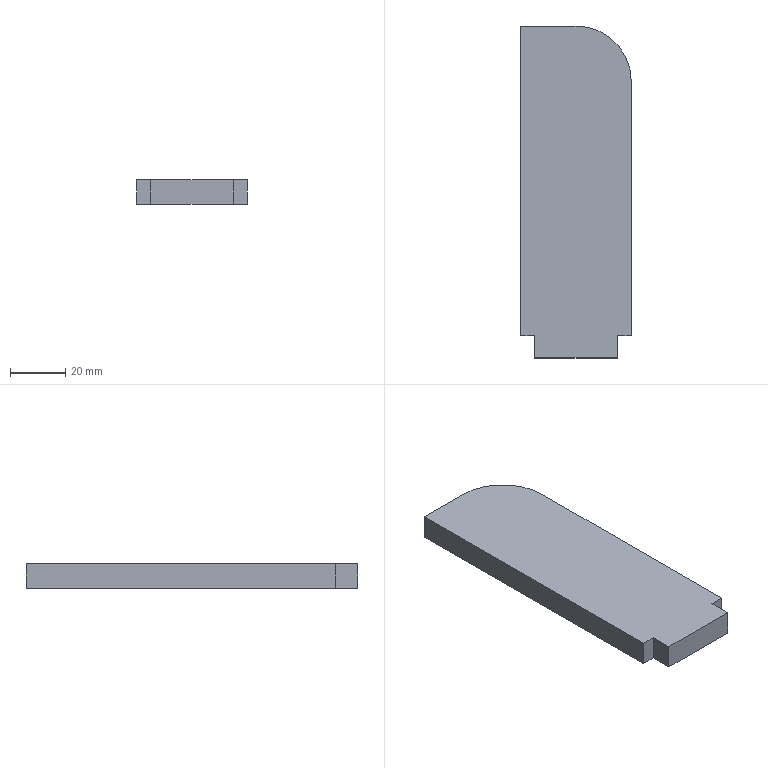Part | SolidWorks | features FlatPattern 1, SMBaseFlange 1, SheetMetal 1 | 1 solid | 11 faces | box 40 x 120 x 9 mm | volume 41707 mm3 | plane 10 | cylinder 1 | commonest cylinder face diameters 40 x1
STEP:
#1=CARTESIAN_POINT('',(0.,100.,0.));
#2=VERTEX_POINT('',#1);
#3=CARTESIAN_POINT('',(-20.,120.,0.));
#4=VERTEX_POINT('',#3);
#5=CARTESIAN_POINT('',(-20.,100.,0.));
#6=DIRECTION('',(0.,0.,1.));
#7=DIRECTION('',(-1.,0.,0.));
#8=AXIS2_PLACEMENT_3D('',#5,#6,#7);
#9=CIRCLE('',#8,20.);
#10=EDGE_CURVE('',#2,#4,#9,.T.);
#11=ORIENTED_EDGE('',*,*,#10,.T.);
#12=CARTESIAN_POINT('',(-20.,120.,9.));
#13=VERTEX_POINT('',#12);
#14=CARTESIAN_POINT('',(-20.,120.,9.));
#15=DIRECTION('',(0.,0.,-1.));
#16=VECTOR('',#15,1000.);
#17=LINE('',#14,#16);
#18=EDGE_CURVE('',#13,#4,#17,.T.);
#19=ORIENTED_EDGE('',*,*,#18,.F.);
#20=CARTESIAN_POINT('',(0.,100.,9.));
#21=VERTEX_POINT('',#20);
#22=CARTESIAN_POINT('',(-20.,100.,9.));
#23=DIRECTION('',(0.,0.,1.));
#24=DIRECTION('',(-1.,0.,0.));
#25=AXIS2_PLACEMENT_3D('',#22,#23,#24);
#26=CIRCLE('',#25,20.);
#27=EDGE_CURVE('',#21,#13,#26,.T.);
#28=ORIENTED_EDGE('',*,*,#27,.F.);
#29=CARTESIAN_POINT('',(0.,100.,9.));
#30=DIRECTION('',(0.,0.,-1.));
#31=VECTOR('',#30,1000.);
#32=LINE('',#29,#31);
#33=EDGE_CURVE('',#21,#2,#32,.T.);
#34=ORIENTED_EDGE('',*,*,#33,.T.);
#35=EDGE_LOOP('',(#11,#19,#28,#34));
#36=FACE_OUTER_BOUND('',#35,.T.);
#37=CARTESIAN_POINT('',(-20.,100.,9.));
#38=DIRECTION('',(0.,0.,-1.));
#39=DIRECTION('',(-1.,0.,0.));
#40=AXIS2_PLACEMENT_3D('',#37,#38,#39);
#41=CYLINDRICAL_SURFACE('',#40,20.);
#42=ADVANCED_FACE('',(#36),#41,.T.);
#43=CARTESIAN_POINT('',(-40.,120.,0.));
#44=VERTEX_POINT('',#43);
#45=CARTESIAN_POINT('',(-20.,120.,0.));
#46=DIRECTION('',(-1.,0.,0.));
#47=VECTOR('',#46,1000.);
#48=LINE('',#45,#47);
#49=EDGE_CURVE('',#4,#44,#48,.T.);
#50=ORIENTED_EDGE('',*,*,#49,.T.);
#51=CARTESIAN_POINT('',(-40.,120.,9.));
#52=VERTEX_POINT('',#51);
#53=CARTESIAN_POINT('',(-40.,120.,9.));
#54=DIRECTION('',(0.,0.,-1.));
#55=VECTOR('',#54,1000.);
#56=LINE('',#53,#55);
#57=EDGE_CURVE('',#52,#44,#56,.T.);
#58=ORIENTED_EDGE('',*,*,#57,.F.);
#59=CARTESIAN_POINT('',(-20.,120.,9.));
#60=DIRECTION('',(-1.,0.,0.));
#61=VECTOR('',#60,1000.);
#62=LINE('',#59,#61);
#63=EDGE_CURVE('',#13,#52,#62,.T.);
#64=ORIENTED_EDGE('',*,*,#63,.F.);
#65=ORIENTED_EDGE('',*,*,#18,.T.);
#66=EDGE_LOOP('',(#50,#58,#64,#65));
#67=FACE_OUTER_BOUND('',#66,.T.);
#68=CARTESIAN_POINT('',(-20.,120.,9.));
#69=DIRECTION('',(0.,-1.,0.));
#70=DIRECTION('',(1.,0.,0.));
#71=AXIS2_PLACEMENT_3D('',#68,#69,#70);
#72=PLANE('',#71);
#73=ADVANCED_FACE('',(#67),#72,.F.);
#74=CARTESIAN_POINT('',(-40.,8.,0.));
#75=VERTEX_POINT('',#74);
#76=CARTESIAN_POINT('',(-40.,120.,0.));
#77=DIRECTION('',(0.,-1.,0.));
#78=VECTOR('',#77,1000.);
#79=LINE('',#76,#78);
#80=EDGE_CURVE('',#44,#75,#79,.T.);
#81=ORIENTED_EDGE('',*,*,#80,.T.);
#82=CARTESIAN_POINT('',(-40.,8.,9.));
#83=VERTEX_POINT('',#82);
#84=CARTESIAN_POINT('',(-40.,8.,9.));
#85=DIRECTION('',(0.,0.,-1.));
#86=VECTOR('',#85,1000.);
#87=LINE('',#84,#86);
#88=EDGE_CURVE('',#83,#75,#87,.T.);
#89=ORIENTED_EDGE('',*,*,#88,.F.);
#90=CARTESIAN_POINT('',(-40.,120.,9.));
#91=DIRECTION('',(0.,-1.,0.));
#92=VECTOR('',#91,1000.);
#93=LINE('',#90,#92);
#94=EDGE_CURVE('',#52,#83,#93,.T.);
#95=ORIENTED_EDGE('',*,*,#94,.F.);
#96=ORIENTED_EDGE('',*,*,#57,.T.);
#97=EDGE_LOOP('',(#81,#89,#95,#96));
#98=FACE_OUTER_BOUND('',#97,.T.);
#99=CARTESIAN_POINT('',(-40.,120.,9.));
#100=DIRECTION('',(1.,0.,0.));
#101=DIRECTION('',(0.,1.,0.));
#102=AXIS2_PLACEMENT_3D('',#99,#100,#101);
#103=PLANE('',#102);
#104=ADVANCED_FACE('',(#98),#103,.F.);
#105=CARTESIAN_POINT('',(-35.,8.,0.));
#106=VERTEX_POINT('',#105);
#107=CARTESIAN_POINT('',(-40.,8.,0.));
#108=DIRECTION('',(1.,0.,0.));
#109=VECTOR('',#108,1000.);
#110=LINE('',#107,#109);
#111=EDGE_CURVE('',#75,#106,#110,.T.);
#112=ORIENTED_EDGE('',*,*,#111,.T.);
#113=CARTESIAN_POINT('',(-35.,8.,9.));
#114=VERTEX_POINT('',#113);
#115=CARTESIAN_POINT('',(-35.,8.,9.));
#116=DIRECTION('',(0.,0.,-1.));
#117=VECTOR('',#116,1000.);
#118=LINE('',#115,#117);
#119=EDGE_CURVE('',#114,#106,#118,.T.);
#120=ORIENTED_EDGE('',*,*,#119,.F.);
#121=CARTESIAN_POINT('',(-40.,8.,9.));
#122=DIRECTION('',(1.,0.,0.));
#123=VECTOR('',#122,1000.);
#124=LINE('',#121,#123);
#125=EDGE_CURVE('',#83,#114,#124,.T.);
#126=ORIENTED_EDGE('',*,*,#125,.F.);
#127=ORIENTED_EDGE('',*,*,#88,.T.);
#128=EDGE_LOOP('',(#112,#120,#126,#127));
#129=FACE_OUTER_BOUND('',#128,.T.);
#130=CARTESIAN_POINT('',(-40.,8.,9.));
#131=DIRECTION('',(0.,1.,0.));
#132=DIRECTION('',(-1.,0.,0.));
#133=AXIS2_PLACEMENT_3D('',#130,#131,#132);
#134=PLANE('',#133);
#135=ADVANCED_FACE('',(#129),#134,.F.);
#136=CARTESIAN_POINT('',(-35.,0.,0.));
#137=VERTEX_POINT('',#136);
#138=CARTESIAN_POINT('',(-35.,8.,0.));
#139=DIRECTION('',(0.,-1.,0.));
#140=VECTOR('',#139,1000.);
#141=LINE('',#138,#140);
#142=EDGE_CURVE('',#106,#137,#141,.T.);
#143=ORIENTED_EDGE('',*,*,#142,.T.);
#144=CARTESIAN_POINT('',(-35.,0.,9.));
#145=VERTEX_POINT('',#144);
#146=CARTESIAN_POINT('',(-35.,0.,9.));
#147=DIRECTION('',(0.,0.,-1.));
#148=VECTOR('',#147,1000.);
#149=LINE('',#146,#148);
#150=EDGE_CURVE('',#145,#137,#149,.T.);
#151=ORIENTED_EDGE('',*,*,#150,.F.);
#152=CARTESIAN_POINT('',(-35.,8.,9.));
#153=DIRECTION('',(0.,-1.,0.));
#154=VECTOR('',#153,1000.);
#155=LINE('',#152,#154);
#156=EDGE_CURVE('',#114,#145,#155,.T.);
#157=ORIENTED_EDGE('',*,*,#156,.F.);
#158=ORIENTED_EDGE('',*,*,#119,.T.);
#159=EDGE_LOOP('',(#143,#151,#157,#158));
#160=FACE_OUTER_BOUND('',#159,.T.);
#161=CARTESIAN_POINT('',(-35.,8.,9.));
#162=DIRECTION('',(1.,0.,0.));
#163=DIRECTION('',(0.,0.,-1.));
#164=AXIS2_PLACEMENT_3D('',#161,#162,#163);
#165=PLANE('',#164);
#166=ADVANCED_FACE('',(#160),#165,.F.);
#167=CARTESIAN_POINT('',(-5.,0.,0.));
#168=VERTEX_POINT('',#167);
#169=CARTESIAN_POINT('',(-35.,0.,0.));
#170=DIRECTION('',(1.,0.,0.));
#171=VECTOR('',#170,1000.);
#172=LINE('',#169,#171);
#173=EDGE_CURVE('',#137,#168,#172,.T.);
#174=ORIENTED_EDGE('',*,*,#173,.T.);
#175=CARTESIAN_POINT('',(-5.,0.,9.));
#176=VERTEX_POINT('',#175);
#177=CARTESIAN_POINT('',(-5.,0.,9.));
#178=DIRECTION('',(0.,0.,-1.));
#179=VECTOR('',#178,1000.);
#180=LINE('',#177,#179);
#181=EDGE_CURVE('',#176,#168,#180,.T.);
#182=ORIENTED_EDGE('',*,*,#181,.F.);
#183=CARTESIAN_POINT('',(-35.,0.,9.));
#184=DIRECTION('',(1.,0.,0.));
#185=VECTOR('',#184,1000.);
#186=LINE('',#183,#185);
#187=EDGE_CURVE('',#145,#176,#186,.T.);
#188=ORIENTED_EDGE('',*,*,#187,.F.);
#189=ORIENTED_EDGE('',*,*,#150,.T.);
#190=EDGE_LOOP('',(#174,#182,#188,#189));
#191=FACE_OUTER_BOUND('',#190,.T.);
#192=CARTESIAN_POINT('',(-35.,0.,9.));
#193=DIRECTION('',(0.,1.,0.));
#194=DIRECTION('',(-1.,0.,0.));
#195=AXIS2_PLACEMENT_3D('',#192,#193,#194);
#196=PLANE('',#195);
#197=ADVANCED_FACE('',(#191),#196,.F.);
#198=CARTESIAN_POINT('',(-5.,8.,0.));
#199=VERTEX_POINT('',#198);
#200=CARTESIAN_POINT('',(-5.,0.,0.));
#201=DIRECTION('',(0.,1.,0.));
#202=VECTOR('',#201,1000.);
#203=LINE('',#200,#202);
#204=EDGE_CURVE('',#168,#199,#203,.T.);
#205=ORIENTED_EDGE('',*,*,#204,.T.);
#206=CARTESIAN_POINT('',(-5.,8.,9.));
#207=VERTEX_POINT('',#206);
#208=CARTESIAN_POINT('',(-5.,8.,9.));
#209=DIRECTION('',(0.,0.,-1.));
#210=VECTOR('',#209,1000.);
#211=LINE('',#208,#210);
#212=EDGE_CURVE('',#207,#199,#211,.T.);
#213=ORIENTED_EDGE('',*,*,#212,.F.);
#214=CARTESIAN_POINT('',(-5.,0.,9.));
#215=DIRECTION('',(0.,1.,0.));
#216=VECTOR('',#215,1000.);
#217=LINE('',#214,#216);
#218=EDGE_CURVE('',#176,#207,#217,.T.);
#219=ORIENTED_EDGE('',*,*,#218,.F.);
#220=ORIENTED_EDGE('',*,*,#181,.T.);
#221=EDGE_LOOP('',(#205,#213,#219,#220));
#222=FACE_OUTER_BOUND('',#221,.T.);
#223=CARTESIAN_POINT('',(-5.,0.,9.));
#224=DIRECTION('',(-1.,0.,0.));
#225=DIRECTION('',(0.,0.,1.));
#226=AXIS2_PLACEMENT_3D('',#223,#224,#225);
#227=PLANE('',#226);
#228=ADVANCED_FACE('',(#222),#227,.F.);
#229=CARTESIAN_POINT('',(0.,8.,0.));
#230=VERTEX_POINT('',#229);
#231=CARTESIAN_POINT('',(-5.,8.,0.));
#232=DIRECTION('',(1.,0.,0.));
#233=VECTOR('',#232,1000.);
#234=LINE('',#231,#233);
#235=EDGE_CURVE('',#199,#230,#234,.T.);
#236=ORIENTED_EDGE('',*,*,#235,.T.);
#237=CARTESIAN_POINT('',(0.,8.,9.));
#238=VERTEX_POINT('',#237);
#239=CARTESIAN_POINT('',(0.,8.,9.));
#240=DIRECTION('',(0.,0.,-1.));
#241=VECTOR('',#240,1000.);
#242=LINE('',#239,#241);
#243=EDGE_CURVE('',#238,#230,#242,.T.);
#244=ORIENTED_EDGE('',*,*,#243,.F.);
#245=CARTESIAN_POINT('',(-5.,8.,9.));
#246=DIRECTION('',(1.,0.,0.));
#247=VECTOR('',#246,1000.);
#248=LINE('',#245,#247);
#249=EDGE_CURVE('',#207,#238,#248,.T.);
#250=ORIENTED_EDGE('',*,*,#249,.F.);
#251=ORIENTED_EDGE('',*,*,#212,.T.);
#252=EDGE_LOOP('',(#236,#244,#250,#251));
#253=FACE_OUTER_BOUND('',#252,.T.);
#254=CARTESIAN_POINT('',(-5.,8.,9.));
#255=DIRECTION('',(0.,1.,0.));
#256=DIRECTION('',(0.,0.,1.));
#257=AXIS2_PLACEMENT_3D('',#254,#255,#256);
#258=PLANE('',#257);
#259=ADVANCED_FACE('',(#253),#258,.F.);
#260=CARTESIAN_POINT('',(0.,8.,0.));
#261=DIRECTION('',(0.,1.,0.));
#262=VECTOR('',#261,1000.);
#263=LINE('',#260,#262);
#264=EDGE_CURVE('',#230,#2,#263,.T.);
#265=ORIENTED_EDGE('',*,*,#264,.T.);
#266=ORIENTED_EDGE('',*,*,#33,.F.);
#267=CARTESIAN_POINT('',(0.,8.,9.));
#268=DIRECTION('',(0.,1.,0.));
#269=VECTOR('',#268,1000.);
#270=LINE('',#267,#269);
#271=EDGE_CURVE('',#238,#21,#270,.T.);
#272=ORIENTED_EDGE('',*,*,#271,.F.);
#273=ORIENTED_EDGE('',*,*,#243,.T.);
#274=EDGE_LOOP('',(#265,#266,#272,#273));
#275=FACE_OUTER_BOUND('',#274,.T.);
#276=CARTESIAN_POINT('',(0.,8.,9.));
#277=DIRECTION('',(-1.,0.,0.));
#278=DIRECTION('',(0.,-1.,0.));
#279=AXIS2_PLACEMENT_3D('',#276,#277,#278);
#280=PLANE('',#279);
#281=ADVANCED_FACE('',(#275),#280,.F.);
#282=ORIENTED_EDGE('',*,*,#27,.T.);
#283=ORIENTED_EDGE('',*,*,#63,.T.);
#284=ORIENTED_EDGE('',*,*,#94,.T.);
#285=ORIENTED_EDGE('',*,*,#125,.T.);
#286=ORIENTED_EDGE('',*,*,#156,.T.);
#287=ORIENTED_EDGE('',*,*,#187,.T.);
#288=ORIENTED_EDGE('',*,*,#218,.T.);
#289=ORIENTED_EDGE('',*,*,#249,.T.);
#290=ORIENTED_EDGE('',*,*,#271,.T.);
#291=EDGE_LOOP('',(#282,#283,#284,#285,#286,#287,#288,#289,#290));
#292=FACE_OUTER_BOUND('',#291,.T.);
#293=CARTESIAN_POINT('',(-20.,100.,9.));
#294=DIRECTION('',(0.,0.,-1.));
#295=DIRECTION('',(-1.,0.,0.));
#296=AXIS2_PLACEMENT_3D('',#293,#294,#295);
#297=PLANE('',#296);
#298=ADVANCED_FACE('',(#292),#297,.F.);
#299=ORIENTED_EDGE('',*,*,#10,.F.);
#300=ORIENTED_EDGE('',*,*,#264,.F.);
#301=ORIENTED_EDGE('',*,*,#235,.F.);
#302=ORIENTED_EDGE('',*,*,#204,.F.);
#303=ORIENTED_EDGE('',*,*,#173,.F.);
#304=ORIENTED_EDGE('',*,*,#142,.F.);
#305=ORIENTED_EDGE('',*,*,#111,.F.);
#306=ORIENTED_EDGE('',*,*,#80,.F.);
#307=ORIENTED_EDGE('',*,*,#49,.F.);
#308=EDGE_LOOP('',(#299,#300,#301,#302,#303,#304,#305,#306,#307));
#309=FACE_OUTER_BOUND('',#308,.T.);
#310=CARTESIAN_POINT('',(-20.,100.,0.));
#311=DIRECTION('',(0.,0.,-1.));
#312=DIRECTION('',(-1.,0.,0.));
#313=AXIS2_PLACEMENT_3D('',#310,#311,#312);
#314=PLANE('',#313);
#315=ADVANCED_FACE('',(#309),#314,.T.);
#316=CLOSED_SHELL('',(#42,#73,#104,#135,#166,#197,#228,#259,#281,#298,#315));
#317=MANIFOLD_SOLID_BREP('',#316);
#318=CARTESIAN_POINT('',(0.,0.,0.));
#319=DIRECTION('',(0.,0.,1.));
#320=DIRECTION('',(1.,0.,0.));
#321=AXIS2_PLACEMENT_3D('',#318,#319,#320);
#322=(LENGTH_UNIT()NAMED_UNIT(*)SI_UNIT(.MILLI.,.METRE.));
#323=UNCERTAINTY_MEASURE_WITH_UNIT(LENGTH_MEASURE(0.00001),#322,'','');
#324=(NAMED_UNIT(*)PLANE_ANGLE_UNIT()SI_UNIT($,.RADIAN.));
#325=(NAMED_UNIT(*)SI_UNIT($,.STERADIAN.)SOLID_ANGLE_UNIT());
#326=(GEOMETRIC_REPRESENTATION_CONTEXT(3)GLOBAL_UNCERTAINTY_ASSIGNED_CONTEXT((#323))GLOBAL_UNIT_ASSIGNED_CONTEXT((#322,#324,#325))REPRESENTATION_CONTEXT('',''));
#327=ADVANCED_BREP_SHAPE_REPRESENTATION('',(#317,#321),#326);